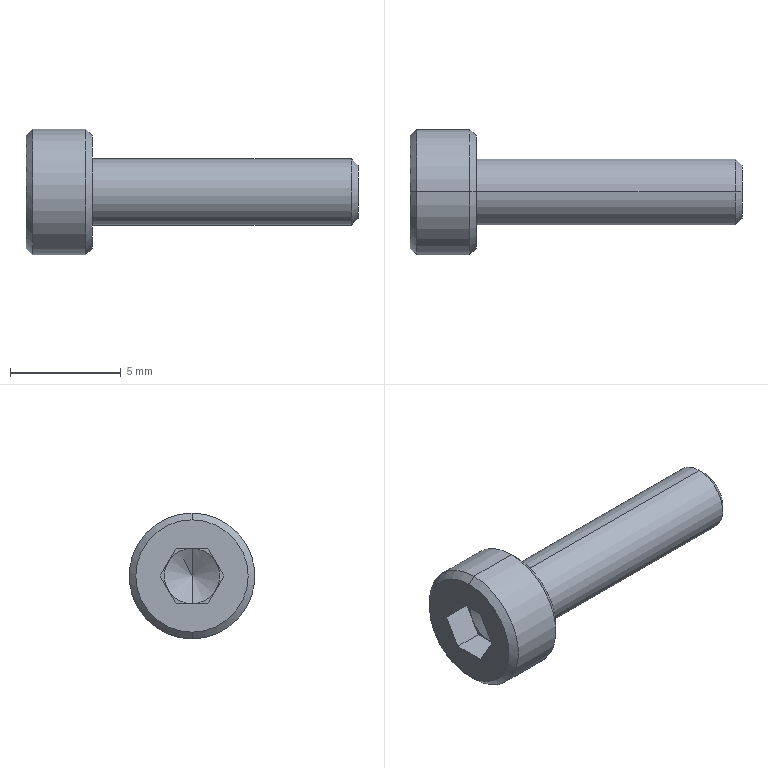Part | STEP file | Hex socket screw Dongming full thread M3-12 A2-70-1 | 1 solid | 27 faces | box 15 x 5.68 x 5.68 mm | volume 150.677 mm3 | plane 15 | cone 8 | cylinder 4 | commonest cylinder face diameters 3 x2 5.68 x2
STEP:
#1=CARTESIAN_POINT('',(15.,0.,-1.2));
#2=VERTEX_POINT('',#1);
#3=CARTESIAN_POINT('',(15.,0.,1.2));
#4=VERTEX_POINT('',#3);
#5=CARTESIAN_POINT('',(15.,0.,0.));
#6=DIRECTION('',(1.,0.,0.));
#7=DIRECTION('',(0.,0.,-1.));
#8=AXIS2_PLACEMENT_3D('',#5,#6,#7);
#9=CIRCLE('',#8,1.2);
#10=EDGE_CURVE('',#2,#4,#9,.T.);
#11=ORIENTED_EDGE('',*,*,#10,.F.);
#12=CARTESIAN_POINT('',(14.7,0.,-1.5));
#13=VERTEX_POINT('',#12);
#14=CARTESIAN_POINT('',(15.,0.,-1.2));
#15=DIRECTION('',(-0.7071,0.,-0.7071));
#16=VECTOR('',#15,1000.);
#17=LINE('',#14,#16);
#18=EDGE_CURVE('',#2,#13,#17,.T.);
#19=ORIENTED_EDGE('',*,*,#18,.T.);
#20=CARTESIAN_POINT('',(14.7,0.,1.5));
#21=VERTEX_POINT('',#20);
#22=CARTESIAN_POINT('',(14.7,0.,0.));
#23=DIRECTION('',(-1.,0.,0.));
#24=DIRECTION('',(0.,0.,-1.));
#25=AXIS2_PLACEMENT_3D('',#22,#23,#24);
#26=CIRCLE('',#25,1.5);
#27=EDGE_CURVE('',#21,#13,#26,.T.);
#28=ORIENTED_EDGE('',*,*,#27,.F.);
#29=CARTESIAN_POINT('',(15.,0.,1.2));
#30=DIRECTION('',(-0.7071,0.,0.7071));
#31=VECTOR('',#30,1000.);
#32=LINE('',#29,#31);
#33=EDGE_CURVE('',#4,#21,#32,.T.);
#34=ORIENTED_EDGE('',*,*,#33,.F.);
#35=EDGE_LOOP('',(#11,#19,#28,#34));
#36=FACE_OUTER_BOUND('',#35,.T.);
#37=CARTESIAN_POINT('',(15.,0.,0.));
#38=DIRECTION('',(-1.,0.,0.));
#39=DIRECTION('',(0.,0.,1.));
#40=AXIS2_PLACEMENT_3D('',#37,#38,#39);
#41=CONICAL_SURFACE('',#40,1.2,0.7854);
#42=ADVANCED_FACE('',(#36),#41,.T.);
#43=CARTESIAN_POINT('',(3.,0.,-2.54));
#44=VERTEX_POINT('',#43);
#45=CARTESIAN_POINT('',(3.,0.,2.54));
#46=VERTEX_POINT('',#45);
#47=CARTESIAN_POINT('',(3.,0.,0.));
#48=DIRECTION('',(1.,0.,0.));
#49=DIRECTION('',(0.,0.,-1.));
#50=AXIS2_PLACEMENT_3D('',#47,#48,#49);
#51=CIRCLE('',#50,2.54);
#52=EDGE_CURVE('',#44,#46,#51,.T.);
#53=ORIENTED_EDGE('',*,*,#52,.F.);
#54=CARTESIAN_POINT('',(2.7,0.,-2.84));
#55=VERTEX_POINT('',#54);
#56=CARTESIAN_POINT('',(3.,0.,-2.54));
#57=DIRECTION('',(-0.7071,0.,-0.7071));
#58=VECTOR('',#57,1000.);
#59=LINE('',#56,#58);
#60=EDGE_CURVE('',#44,#55,#59,.T.);
#61=ORIENTED_EDGE('',*,*,#60,.T.);
#62=CARTESIAN_POINT('',(2.7,0.,2.84));
#63=VERTEX_POINT('',#62);
#64=CARTESIAN_POINT('',(2.7,0.,0.));
#65=DIRECTION('',(-1.,0.,0.));
#66=DIRECTION('',(0.,0.,-1.));
#67=AXIS2_PLACEMENT_3D('',#64,#65,#66);
#68=CIRCLE('',#67,2.84);
#69=EDGE_CURVE('',#63,#55,#68,.T.);
#70=ORIENTED_EDGE('',*,*,#69,.F.);
#71=CARTESIAN_POINT('',(3.,0.,2.54));
#72=DIRECTION('',(-0.7071,0.,0.7071));
#73=VECTOR('',#72,1000.);
#74=LINE('',#71,#73);
#75=EDGE_CURVE('',#46,#63,#74,.T.);
#76=ORIENTED_EDGE('',*,*,#75,.F.);
#77=EDGE_LOOP('',(#53,#61,#70,#76));
#78=FACE_OUTER_BOUND('',#77,.T.);
#79=CARTESIAN_POINT('',(3.,0.,0.));
#80=DIRECTION('',(-1.,0.,0.));
#81=DIRECTION('',(0.,0.,1.));
#82=AXIS2_PLACEMENT_3D('',#79,#80,#81);
#83=CONICAL_SURFACE('',#82,2.54,0.7854);
#84=ADVANCED_FACE('',(#78),#83,.T.);
#85=CARTESIAN_POINT('',(0.,0.,2.54));
#86=VERTEX_POINT('',#85);
#87=CARTESIAN_POINT('',(0.,0.,-2.54));
#88=VERTEX_POINT('',#87);
#89=CARTESIAN_POINT('',(0.,0.,0.));
#90=DIRECTION('',(-1.,0.,0.));
#91=DIRECTION('',(0.,0.,-1.));
#92=AXIS2_PLACEMENT_3D('',#89,#90,#91);
#93=CIRCLE('',#92,2.54);
#94=EDGE_CURVE('',#86,#88,#93,.T.);
#95=ORIENTED_EDGE('',*,*,#94,.F.);
#96=CARTESIAN_POINT('',(0.3,0.,2.84));
#97=VERTEX_POINT('',#96);
#98=CARTESIAN_POINT('',(0.3,0.,2.84));
#99=DIRECTION('',(0.7071,0.,0.7071));
#100=VECTOR('',#99,1000.);
#101=LINE('',#98,#100);
#102=EDGE_CURVE('',#86,#97,#101,.T.);
#103=ORIENTED_EDGE('',*,*,#102,.T.);
#104=CARTESIAN_POINT('',(0.3,0.,-2.84));
#105=VERTEX_POINT('',#104);
#106=CARTESIAN_POINT('',(0.3,0.,0.));
#107=DIRECTION('',(1.,0.,0.));
#108=DIRECTION('',(0.,0.,-1.));
#109=AXIS2_PLACEMENT_3D('',#106,#107,#108);
#110=CIRCLE('',#109,2.84);
#111=EDGE_CURVE('',#105,#97,#110,.T.);
#112=ORIENTED_EDGE('',*,*,#111,.F.);
#113=CARTESIAN_POINT('',(0.3,0.,-2.84));
#114=DIRECTION('',(0.7071,0.,-0.7071));
#115=VECTOR('',#114,1000.);
#116=LINE('',#113,#115);
#117=EDGE_CURVE('',#88,#105,#116,.T.);
#118=ORIENTED_EDGE('',*,*,#117,.F.);
#119=EDGE_LOOP('',(#95,#103,#112,#118));
#120=FACE_OUTER_BOUND('',#119,.T.);
#121=CARTESIAN_POINT('',(0.3,0.,0.));
#122=DIRECTION('',(1.,0.,0.));
#123=DIRECTION('',(0.,0.,-1.));
#124=AXIS2_PLACEMENT_3D('',#121,#122,#123);
#125=CONICAL_SURFACE('',#124,2.84,0.7854);
#126=ADVANCED_FACE('',(#120),#125,.T.);
#127=CARTESIAN_POINT('',(2.022,0.,0.));
#128=VERTEX_POINT('',#127);
#129=CARTESIAN_POINT('',(1.3,0.,1.25));
#130=VERTEX_POINT('',#129);
#131=CARTESIAN_POINT('',(2.022,0.,0.));
#132=DIRECTION('',(-0.5,0.,0.866));
#133=VECTOR('',#132,1000.);
#134=LINE('',#131,#133);
#135=EDGE_CURVE('',#128,#130,#134,.T.);
#136=ORIENTED_EDGE('',*,*,#135,.F.);
#137=CARTESIAN_POINT('',(1.3,0.,-1.25));
#138=VERTEX_POINT('',#137);
#139=CARTESIAN_POINT('',(2.022,0.,0.));
#140=DIRECTION('',(-0.5,0.,-0.866));
#141=VECTOR('',#140,1000.);
#142=LINE('',#139,#141);
#143=EDGE_CURVE('',#128,#138,#142,.T.);
#144=ORIENTED_EDGE('',*,*,#143,.T.);
#145=CARTESIAN_POINT('',(1.3,-1.083,-0.625));
#146=VERTEX_POINT('',#145);
#147=CARTESIAN_POINT('',(1.3,0.,0.));
#148=DIRECTION('',(-1.,0.,0.));
#149=DIRECTION('',(0.,0.,1.));
#150=AXIS2_PLACEMENT_3D('',#147,#148,#149);
#151=CIRCLE('',#150,1.25);
#152=EDGE_CURVE('',#138,#146,#151,.T.);
#153=ORIENTED_EDGE('',*,*,#152,.T.);
#154=CARTESIAN_POINT('',(1.3,-1.083,0.625));
#155=VERTEX_POINT('',#154);
#156=CARTESIAN_POINT('',(1.3,0.,0.));
#157=DIRECTION('',(-1.,0.,0.));
#158=DIRECTION('',(0.,0.,1.));
#159=AXIS2_PLACEMENT_3D('',#156,#157,#158);
#160=CIRCLE('',#159,1.25);
#161=EDGE_CURVE('',#146,#155,#160,.T.);
#162=ORIENTED_EDGE('',*,*,#161,.T.);
#163=CARTESIAN_POINT('',(1.3,0.,0.));
#164=DIRECTION('',(-1.,0.,0.));
#165=DIRECTION('',(0.,0.,1.));
#166=AXIS2_PLACEMENT_3D('',#163,#164,#165);
#167=CIRCLE('',#166,1.25);
#168=EDGE_CURVE('',#155,#130,#167,.T.);
#169=ORIENTED_EDGE('',*,*,#168,.T.);
#170=EDGE_LOOP('',(#136,#144,#153,#162,#169));
#171=FACE_OUTER_BOUND('',#170,.T.);
#172=CARTESIAN_POINT('',(-997.978,0.,0.));
#173=DIRECTION('',(-1.,0.,0.));
#174=DIRECTION('',(0.,0.,1.));
#175=AXIS2_PLACEMENT_3D('',#172,#173,#174);
#176=CONICAL_SURFACE('',#175,1732.051,1.047);
#177=ADVANCED_FACE('',(#171),#176,.F.);
#178=ORIENTED_EDGE('',*,*,#27,.T.);
#179=CARTESIAN_POINT('',(3.,0.,-1.5));
#180=VERTEX_POINT('',#179);
#181=CARTESIAN_POINT('',(15.,0.,-1.5));
#182=DIRECTION('',(-1.,0.,0.));
#183=VECTOR('',#182,1000.);
#184=LINE('',#181,#183);
#185=EDGE_CURVE('',#13,#180,#184,.T.);
#186=ORIENTED_EDGE('',*,*,#185,.T.);
#187=CARTESIAN_POINT('',(3.,0.,1.5));
#188=VERTEX_POINT('',#187);
#189=CARTESIAN_POINT('',(3.,0.,0.));
#190=DIRECTION('',(1.,0.,0.));
#191=DIRECTION('',(0.,0.,-1.));
#192=AXIS2_PLACEMENT_3D('',#189,#190,#191);
#193=CIRCLE('',#192,1.5);
#194=EDGE_CURVE('',#180,#188,#193,.T.);
#195=ORIENTED_EDGE('',*,*,#194,.T.);
#196=CARTESIAN_POINT('',(15.,0.,1.5));
#197=DIRECTION('',(-1.,0.,0.));
#198=VECTOR('',#197,1000.);
#199=LINE('',#196,#198);
#200=EDGE_CURVE('',#21,#188,#199,.T.);
#201=ORIENTED_EDGE('',*,*,#200,.F.);
#202=EDGE_LOOP('',(#178,#186,#195,#201));
#203=FACE_OUTER_BOUND('',#202,.T.);
#204=CARTESIAN_POINT('',(15.,0.,0.));
#205=DIRECTION('',(-1.,0.,0.));
#206=DIRECTION('',(0.,0.,1.));
#207=AXIS2_PLACEMENT_3D('',#204,#205,#206);
#208=CYLINDRICAL_SURFACE('',#207,1.5);
#209=ADVANCED_FACE('',(#203),#208,.T.);
#210=ORIENTED_EDGE('',*,*,#69,.T.);
#211=CARTESIAN_POINT('',(3.,0.,-2.84));
#212=DIRECTION('',(-1.,0.,0.));
#213=VECTOR('',#212,1000.);
#214=LINE('',#211,#213);
#215=EDGE_CURVE('',#55,#105,#214,.T.);
#216=ORIENTED_EDGE('',*,*,#215,.T.);
#217=ORIENTED_EDGE('',*,*,#111,.T.);
#218=CARTESIAN_POINT('',(3.,0.,2.84));
#219=DIRECTION('',(-1.,0.,0.));
#220=VECTOR('',#219,1000.);
#221=LINE('',#218,#220);
#222=EDGE_CURVE('',#63,#97,#221,.T.);
#223=ORIENTED_EDGE('',*,*,#222,.F.);
#224=EDGE_LOOP('',(#210,#216,#217,#223));
#225=FACE_OUTER_BOUND('',#224,.T.);
#226=CARTESIAN_POINT('',(3.,0.,0.));
#227=DIRECTION('',(-1.,0.,0.));
#228=DIRECTION('',(0.,0.,1.));
#229=AXIS2_PLACEMENT_3D('',#226,#227,#228);
#230=CYLINDRICAL_SURFACE('',#229,2.84);
#231=ADVANCED_FACE('',(#225),#230,.T.);
#232=CARTESIAN_POINT('',(1.3,1.083,0.625));
#233=VERTEX_POINT('',#232);
#234=CARTESIAN_POINT('',(1.3,0.,0.));
#235=DIRECTION('',(-1.,0.,0.));
#236=DIRECTION('',(0.,0.,1.));
#237=AXIS2_PLACEMENT_3D('',#234,#235,#236);
#238=CIRCLE('',#237,1.25);
#239=EDGE_CURVE('',#130,#233,#238,.T.);
#240=ORIENTED_EDGE('',*,*,#239,.F.);
#241=CARTESIAN_POINT('',(1.3,0.7217,1.25));
#242=VERTEX_POINT('',#241);
#243=CARTESIAN_POINT('',(1.3,-0.7217,1.25));
#244=DIRECTION('',(0.,1.,0.));
#245=VECTOR('',#244,1000.);
#246=LINE('',#243,#245);
#247=EDGE_CURVE('',#130,#242,#246,.T.);
#248=ORIENTED_EDGE('',*,*,#247,.T.);
#249=CARTESIAN_POINT('',(1.3,0.7217,1.25));
#250=DIRECTION('',(0.,0.5,-0.866));
#251=VECTOR('',#250,1000.);
#252=LINE('',#249,#251);
#253=EDGE_CURVE('',#242,#233,#252,.T.);
#254=ORIENTED_EDGE('',*,*,#253,.T.);
#255=EDGE_LOOP('',(#240,#248,#254));
#256=FACE_OUTER_BOUND('',#255,.T.);
#257=CARTESIAN_POINT('',(1.3,0.,0.));
#258=DIRECTION('',(-1.,0.,0.));
#259=DIRECTION('',(0.,0.,1.));
#260=AXIS2_PLACEMENT_3D('',#257,#258,#259);
#261=PLANE('',#260);
#262=ADVANCED_FACE('',(#256),#261,.T.);
#263=CARTESIAN_POINT('',(1.3,1.083,-0.625));
#264=VERTEX_POINT('',#263);
#265=CARTESIAN_POINT('',(1.3,0.,0.));
#266=DIRECTION('',(-1.,0.,0.));
#267=DIRECTION('',(0.,0.,1.));
#268=AXIS2_PLACEMENT_3D('',#265,#266,#267);
#269=CIRCLE('',#268,1.25);
#270=EDGE_CURVE('',#233,#264,#269,.T.);
#271=ORIENTED_EDGE('',*,*,#270,.F.);
#272=CARTESIAN_POINT('',(1.3,1.443,0.));
#273=VERTEX_POINT('',#272);
#274=CARTESIAN_POINT('',(1.3,0.7217,1.25));
#275=DIRECTION('',(0.,0.5,-0.866));
#276=VECTOR('',#275,1000.);
#277=LINE('',#274,#276);
#278=EDGE_CURVE('',#233,#273,#277,.T.);
#279=ORIENTED_EDGE('',*,*,#278,.T.);
#280=CARTESIAN_POINT('',(1.3,1.443,0.));
#281=DIRECTION('',(0.,-0.5,-0.866));
#282=VECTOR('',#281,1000.);
#283=LINE('',#280,#282);
#284=EDGE_CURVE('',#273,#264,#283,.T.);
#285=ORIENTED_EDGE('',*,*,#284,.T.);
#286=EDGE_LOOP('',(#271,#279,#285));
#287=FACE_OUTER_BOUND('',#286,.T.);
#288=CARTESIAN_POINT('',(1.3,0.,0.));
#289=DIRECTION('',(-1.,0.,0.));
#290=DIRECTION('',(0.,0.,1.));
#291=AXIS2_PLACEMENT_3D('',#288,#289,#290);
#292=PLANE('',#291);
#293=ADVANCED_FACE('',(#287),#292,.T.);
#294=CARTESIAN_POINT('',(1.3,0.,0.));
#295=DIRECTION('',(-1.,0.,0.));
#296=DIRECTION('',(0.,0.,1.));
#297=AXIS2_PLACEMENT_3D('',#294,#295,#296);
#298=CIRCLE('',#297,1.25);
#299=EDGE_CURVE('',#264,#138,#298,.T.);
#300=ORIENTED_EDGE('',*,*,#299,.F.);
#301=CARTESIAN_POINT('',(1.3,0.7217,-1.25));
#302=VERTEX_POINT('',#301);
#303=CARTESIAN_POINT('',(1.3,1.443,0.));
#304=DIRECTION('',(0.,-0.5,-0.866));
#305=VECTOR('',#304,1000.);
#306=LINE('',#303,#305);
#307=EDGE_CURVE('',#264,#302,#306,.T.);
#308=ORIENTED_EDGE('',*,*,#307,.T.);
#309=CARTESIAN_POINT('',(1.3,0.7217,-1.25));
#310=DIRECTION('',(0.,-1.,0.));
#311=VECTOR('',#310,1000.);
#312=LINE('',#309,#311);
#313=EDGE_CURVE('',#302,#138,#312,.T.);
#314=ORIENTED_EDGE('',*,*,#313,.T.);
#315=EDGE_LOOP('',(#300,#308,#314));
#316=FACE_OUTER_BOUND('',#315,.T.);
#317=CARTESIAN_POINT('',(1.3,0.,0.));
#318=DIRECTION('',(-1.,0.,0.));
#319=DIRECTION('',(0.,0.,1.));
#320=AXIS2_PLACEMENT_3D('',#317,#318,#319);
#321=PLANE('',#320);
#322=ADVANCED_FACE('',(#316),#321,.T.);
#323=ORIENTED_EDGE('',*,*,#152,.F.);
#324=CARTESIAN_POINT('',(1.3,-0.7217,-1.25));
#325=VERTEX_POINT('',#324);
#326=CARTESIAN_POINT('',(1.3,0.7217,-1.25));
#327=DIRECTION('',(0.,-1.,0.));
#328=VECTOR('',#327,1000.);
#329=LINE('',#326,#328);
#330=EDGE_CURVE('',#138,#325,#329,.T.);
#331=ORIENTED_EDGE('',*,*,#330,.T.);
#332=CARTESIAN_POINT('',(1.3,-0.7217,-1.25));
#333=DIRECTION('',(0.,-0.5,0.866));
#334=VECTOR('',#333,1000.);
#335=LINE('',#332,#334);
#336=EDGE_CURVE('',#325,#146,#335,.T.);
#337=ORIENTED_EDGE('',*,*,#336,.T.);
#338=EDGE_LOOP('',(#323,#331,#337));
#339=FACE_OUTER_BOUND('',#338,.T.);
#340=CARTESIAN_POINT('',(1.3,0.,0.));
#341=DIRECTION('',(-1.,0.,0.));
#342=DIRECTION('',(0.,0.,1.));
#343=AXIS2_PLACEMENT_3D('',#340,#341,#342);
#344=PLANE('',#343);
#345=ADVANCED_FACE('',(#339),#344,.T.);
#346=ORIENTED_EDGE('',*,*,#161,.F.);
#347=CARTESIAN_POINT('',(1.3,-1.443,0.));
#348=VERTEX_POINT('',#347);
#349=CARTESIAN_POINT('',(1.3,-0.7217,-1.25));
#350=DIRECTION('',(0.,-0.5,0.866));
#351=VECTOR('',#350,1000.);
#352=LINE('',#349,#351);
#353=EDGE_CURVE('',#146,#348,#352,.T.);
#354=ORIENTED_EDGE('',*,*,#353,.T.);
#355=CARTESIAN_POINT('',(1.3,-1.443,0.));
#356=DIRECTION('',(0.,0.5,0.866));
#357=VECTOR('',#356,1000.);
#358=LINE('',#355,#357);
#359=EDGE_CURVE('',#348,#155,#358,.T.);
#360=ORIENTED_EDGE('',*,*,#359,.T.);
#361=EDGE_LOOP('',(#346,#354,#360));
#362=FACE_OUTER_BOUND('',#361,.T.);
#363=CARTESIAN_POINT('',(1.3,0.,0.));
#364=DIRECTION('',(-1.,0.,0.));
#365=DIRECTION('',(0.,0.,1.));
#366=AXIS2_PLACEMENT_3D('',#363,#364,#365);
#367=PLANE('',#366);
#368=ADVANCED_FACE('',(#362),#367,.T.);
#369=ORIENTED_EDGE('',*,*,#215,.F.);
#370=CARTESIAN_POINT('',(2.7,0.,0.));
#371=DIRECTION('',(-1.,0.,0.));
#372=DIRECTION('',(0.,0.,-1.));
#373=AXIS2_PLACEMENT_3D('',#370,#371,#372);
#374=CIRCLE('',#373,2.84);
#375=EDGE_CURVE('',#55,#63,#374,.T.);
#376=ORIENTED_EDGE('',*,*,#375,.T.);
#377=ORIENTED_EDGE('',*,*,#222,.T.);
#378=CARTESIAN_POINT('',(0.3,0.,0.));
#379=DIRECTION('',(1.,0.,0.));
#380=DIRECTION('',(0.,0.,-1.));
#381=AXIS2_PLACEMENT_3D('',#378,#379,#380);
#382=CIRCLE('',#381,2.84);
#383=EDGE_CURVE('',#97,#105,#382,.T.);
#384=ORIENTED_EDGE('',*,*,#383,.T.);
#385=EDGE_LOOP('',(#369,#376,#377,#384));
#386=FACE_OUTER_BOUND('',#385,.T.);
#387=CARTESIAN_POINT('',(3.,0.,0.));
#388=DIRECTION('',(-1.,0.,0.));
#389=DIRECTION('',(0.,0.,1.));
#390=AXIS2_PLACEMENT_3D('',#387,#388,#389);
#391=CYLINDRICAL_SURFACE('',#390,2.84);
#392=ADVANCED_FACE('',(#386),#391,.T.);
#393=CARTESIAN_POINT('',(3.,0.,0.));
#394=DIRECTION('',(1.,0.,0.));
#395=DIRECTION('',(0.,0.,-1.));
#396=AXIS2_PLACEMENT_3D('',#393,#394,#395);
#397=CIRCLE('',#396,2.54);
#398=EDGE_CURVE('',#46,#44,#397,.T.);
#399=ORIENTED_EDGE('',*,*,#398,.T.);
#400=ORIENTED_EDGE('',*,*,#52,.T.);
#401=EDGE_LOOP('',(#399,#400));
#402=FACE_OUTER_BOUND('',#401,.T.);
#403=CARTESIAN_POINT('',(3.,0.,0.));
#404=DIRECTION('',(1.,0.,0.));
#405=DIRECTION('',(0.,0.,-1.));
#406=AXIS2_PLACEMENT_3D('',#403,#404,#405);
#407=CIRCLE('',#406,1.5);
#408=EDGE_CURVE('',#188,#180,#407,.T.);
#409=ORIENTED_EDGE('',*,*,#408,.F.);
#410=ORIENTED_EDGE('',*,*,#194,.F.);
#411=EDGE_LOOP('',(#409,#410));
#412=FACE_BOUND('',#411,.T.);
#413=CARTESIAN_POINT('',(3.,0.,0.));
#414=DIRECTION('',(1.,0.,0.));
#415=DIRECTION('',(0.,0.,-1.));
#416=AXIS2_PLACEMENT_3D('',#413,#414,#415);
#417=PLANE('',#416);
#418=ADVANCED_FACE('',(#402,#412),#417,.T.);
#419=CARTESIAN_POINT('',(0.,0.,0.));
#420=DIRECTION('',(-1.,0.,0.));
#421=DIRECTION('',(0.,0.,-1.));
#422=AXIS2_PLACEMENT_3D('',#419,#420,#421);
#423=CIRCLE('',#422,2.54);
#424=EDGE_CURVE('',#88,#86,#423,.T.);
#425=ORIENTED_EDGE('',*,*,#424,.T.);
#426=ORIENTED_EDGE('',*,*,#94,.T.);
#427=EDGE_LOOP('',(#425,#426));
#428=FACE_OUTER_BOUND('',#427,.T.);
#429=CARTESIAN_POINT('',(0.,1.443,0.));
#430=VERTEX_POINT('',#429);
#431=CARTESIAN_POINT('',(0.,0.7217,-1.25));
#432=VERTEX_POINT('',#431);
#433=CARTESIAN_POINT('',(0.,1.443,0.));
#434=DIRECTION('',(0.,-0.5,-0.866));
#435=VECTOR('',#434,1000.);
#436=LINE('',#433,#435);
#437=EDGE_CURVE('',#430,#432,#436,.T.);
#438=ORIENTED_EDGE('',*,*,#437,.F.);
#439=CARTESIAN_POINT('',(0.,0.7217,1.25));
#440=VERTEX_POINT('',#439);
#441=CARTESIAN_POINT('',(0.,0.7217,1.25));
#442=DIRECTION('',(0.,0.5,-0.866));
#443=VECTOR('',#442,1000.);
#444=LINE('',#441,#443);
#445=EDGE_CURVE('',#440,#430,#444,.T.);
#446=ORIENTED_EDGE('',*,*,#445,.F.);
#447=CARTESIAN_POINT('',(0.,-0.7217,1.25));
#448=VERTEX_POINT('',#447);
#449=CARTESIAN_POINT('',(0.,-0.7217,1.25));
#450=DIRECTION('',(0.,1.,0.));
#451=VECTOR('',#450,1000.);
#452=LINE('',#449,#451);
#453=EDGE_CURVE('',#448,#440,#452,.T.);
#454=ORIENTED_EDGE('',*,*,#453,.F.);
#455=CARTESIAN_POINT('',(0.,-1.443,0.));
#456=VERTEX_POINT('',#455);
#457=CARTESIAN_POINT('',(0.,-1.443,0.));
#458=DIRECTION('',(0.,0.5,0.866));
#459=VECTOR('',#458,1000.);
#460=LINE('',#457,#459);
#461=EDGE_CURVE('',#456,#448,#460,.T.);
#462=ORIENTED_EDGE('',*,*,#461,.F.);
#463=CARTESIAN_POINT('',(0.,-0.7217,-1.25));
#464=VERTEX_POINT('',#463);
#465=CARTESIAN_POINT('',(0.,-0.7217,-1.25));
#466=DIRECTION('',(0.,-0.5,0.866));
#467=VECTOR('',#466,1000.);
#468=LINE('',#465,#467);
#469=EDGE_CURVE('',#464,#456,#468,.T.);
#470=ORIENTED_EDGE('',*,*,#469,.F.);
#471=CARTESIAN_POINT('',(0.,0.7217,-1.25));
#472=DIRECTION('',(0.,-1.,0.));
#473=VECTOR('',#472,1000.);
#474=LINE('',#471,#473);
#475=EDGE_CURVE('',#432,#464,#474,.T.);
#476=ORIENTED_EDGE('',*,*,#475,.F.);
#477=EDGE_LOOP('',(#438,#446,#454,#462,#470,#476));
#478=FACE_BOUND('',#477,.T.);
#479=CARTESIAN_POINT('',(0.,0.,0.));
#480=DIRECTION('',(1.,0.,0.));
#481=DIRECTION('',(0.,0.,-1.));
#482=AXIS2_PLACEMENT_3D('',#479,#480,#481);
#483=PLANE('',#482);
#484=ADVANCED_FACE('',(#428,#478),#483,.F.);
#485=ORIENTED_EDGE('',*,*,#185,.F.);
#486=CARTESIAN_POINT('',(14.7,0.,0.));
#487=DIRECTION('',(-1.,0.,0.));
#488=DIRECTION('',(0.,0.,-1.));
#489=AXIS2_PLACEMENT_3D('',#486,#487,#488);
#490=CIRCLE('',#489,1.5);
#491=EDGE_CURVE('',#13,#21,#490,.T.);
#492=ORIENTED_EDGE('',*,*,#491,.T.);
#493=ORIENTED_EDGE('',*,*,#200,.T.);
#494=ORIENTED_EDGE('',*,*,#408,.T.);
#495=EDGE_LOOP('',(#485,#492,#493,#494));
#496=FACE_OUTER_BOUND('',#495,.T.);
#497=CARTESIAN_POINT('',(15.,0.,0.));
#498=DIRECTION('',(-1.,0.,0.));
#499=DIRECTION('',(0.,0.,1.));
#500=AXIS2_PLACEMENT_3D('',#497,#498,#499);
#501=CYLINDRICAL_SURFACE('',#500,1.5);
#502=ADVANCED_FACE('',(#496),#501,.T.);
#503=CARTESIAN_POINT('',(15.,0.,0.));
#504=DIRECTION('',(1.,0.,0.));
#505=DIRECTION('',(0.,0.,-1.));
#506=AXIS2_PLACEMENT_3D('',#503,#504,#505);
#507=CIRCLE('',#506,1.2);
#508=EDGE_CURVE('',#4,#2,#507,.T.);
#509=ORIENTED_EDGE('',*,*,#508,.T.);
#510=ORIENTED_EDGE('',*,*,#10,.T.);
#511=EDGE_LOOP('',(#509,#510));
#512=FACE_OUTER_BOUND('',#511,.T.);
#513=CARTESIAN_POINT('',(15.,0.,0.));
#514=DIRECTION('',(1.,0.,0.));
#515=DIRECTION('',(0.,0.,-1.));
#516=AXIS2_PLACEMENT_3D('',#513,#514,#515);
#517=PLANE('',#516);
#518=ADVANCED_FACE('',(#512),#517,.T.);
#519=ORIENTED_EDGE('',*,*,#445,.T.);
#520=CARTESIAN_POINT('',(1.3,1.443,0.));
#521=DIRECTION('',(-1.,0.,0.));
#522=VECTOR('',#521,1000.);
#523=LINE('',#520,#522);
#524=EDGE_CURVE('',#273,#430,#523,.T.);
#525=ORIENTED_EDGE('',*,*,#524,.F.);
#526=ORIENTED_EDGE('',*,*,#278,.F.);
#527=ORIENTED_EDGE('',*,*,#253,.F.);
#528=CARTESIAN_POINT('',(1.3,0.7217,1.25));
#529=DIRECTION('',(-1.,0.,0.));
#530=VECTOR('',#529,1000.);
#531=LINE('',#528,#530);
#532=EDGE_CURVE('',#242,#440,#531,.T.);
#533=ORIENTED_EDGE('',*,*,#532,.T.);
#534=EDGE_LOOP('',(#519,#525,#526,#527,#533));
#535=FACE_OUTER_BOUND('',#534,.T.);
#536=CARTESIAN_POINT('',(1.3,0.7217,1.25));
#537=DIRECTION('',(0.,0.866,0.5));
#538=DIRECTION('',(0.,-0.5,0.866));
#539=AXIS2_PLACEMENT_3D('',#536,#537,#538);
#540=PLANE('',#539);
#541=ADVANCED_FACE('',(#535),#540,.F.);
#542=ORIENTED_EDGE('',*,*,#453,.T.);
#543=ORIENTED_EDGE('',*,*,#532,.F.);
#544=ORIENTED_EDGE('',*,*,#247,.F.);
#545=CARTESIAN_POINT('',(1.3,-0.7217,1.25));
#546=VERTEX_POINT('',#545);
#547=CARTESIAN_POINT('',(1.3,-0.7217,1.25));
#548=DIRECTION('',(0.,1.,0.));
#549=VECTOR('',#548,1000.);
#550=LINE('',#547,#549);
#551=EDGE_CURVE('',#546,#130,#550,.T.);
#552=ORIENTED_EDGE('',*,*,#551,.F.);
#553=CARTESIAN_POINT('',(1.3,-0.7217,1.25));
#554=DIRECTION('',(-1.,0.,0.));
#555=VECTOR('',#554,1000.);
#556=LINE('',#553,#555);
#557=EDGE_CURVE('',#546,#448,#556,.T.);
#558=ORIENTED_EDGE('',*,*,#557,.T.);
#559=EDGE_LOOP('',(#542,#543,#544,#552,#558));
#560=FACE_OUTER_BOUND('',#559,.T.);
#561=CARTESIAN_POINT('',(1.3,-0.7217,1.25));
#562=DIRECTION('',(0.,0.,1.));
#563=DIRECTION('',(0.,-1.,0.));
#564=AXIS2_PLACEMENT_3D('',#561,#562,#563);
#565=PLANE('',#564);
#566=ADVANCED_FACE('',(#560),#565,.F.);
#567=ORIENTED_EDGE('',*,*,#461,.T.);
#568=ORIENTED_EDGE('',*,*,#557,.F.);
#569=CARTESIAN_POINT('',(1.3,-1.443,0.));
#570=DIRECTION('',(0.,0.5,0.866));
#571=VECTOR('',#570,1000.);
#572=LINE('',#569,#571);
#573=EDGE_CURVE('',#155,#546,#572,.T.);
#574=ORIENTED_EDGE('',*,*,#573,.F.);
#575=ORIENTED_EDGE('',*,*,#359,.F.);
#576=CARTESIAN_POINT('',(1.3,-1.443,0.));
#577=DIRECTION('',(-1.,0.,0.));
#578=VECTOR('',#577,1000.);
#579=LINE('',#576,#578);
#580=EDGE_CURVE('',#348,#456,#579,.T.);
#581=ORIENTED_EDGE('',*,*,#580,.T.);
#582=EDGE_LOOP('',(#567,#568,#574,#575,#581));
#583=FACE_OUTER_BOUND('',#582,.T.);
#584=CARTESIAN_POINT('',(1.3,-1.443,0.));
#585=DIRECTION('',(0.,-0.866,0.5));
#586=DIRECTION('',(0.,-0.5,-0.866));
#587=AXIS2_PLACEMENT_3D('',#584,#585,#586);
#588=PLANE('',#587);
#589=ADVANCED_FACE('',(#583),#588,.F.);
#590=ORIENTED_EDGE('',*,*,#469,.T.);
#591=ORIENTED_EDGE('',*,*,#580,.F.);
#592=ORIENTED_EDGE('',*,*,#353,.F.);
#593=ORIENTED_EDGE('',*,*,#336,.F.);
#594=CARTESIAN_POINT('',(1.3,-0.7217,-1.25));
#595=DIRECTION('',(-1.,0.,0.));
#596=VECTOR('',#595,1000.);
#597=LINE('',#594,#596);
#598=EDGE_CURVE('',#325,#464,#597,.T.);
#599=ORIENTED_EDGE('',*,*,#598,.T.);
#600=EDGE_LOOP('',(#590,#591,#592,#593,#599));
#601=FACE_OUTER_BOUND('',#600,.T.);
#602=CARTESIAN_POINT('',(1.3,-0.7217,-1.25));
#603=DIRECTION('',(0.,-0.866,-0.5));
#604=DIRECTION('',(0.,0.5,-0.866));
#605=AXIS2_PLACEMENT_3D('',#602,#603,#604);
#606=PLANE('',#605);
#607=ADVANCED_FACE('',(#601),#606,.F.);
#608=ORIENTED_EDGE('',*,*,#475,.T.);
#609=ORIENTED_EDGE('',*,*,#598,.F.);
#610=ORIENTED_EDGE('',*,*,#330,.F.);
#611=ORIENTED_EDGE('',*,*,#313,.F.);
#612=CARTESIAN_POINT('',(1.3,0.7217,-1.25));
#613=DIRECTION('',(-1.,0.,0.));
#614=VECTOR('',#613,1000.);
#615=LINE('',#612,#614);
#616=EDGE_CURVE('',#302,#432,#615,.T.);
#617=ORIENTED_EDGE('',*,*,#616,.T.);
#618=EDGE_LOOP('',(#608,#609,#610,#611,#617));
#619=FACE_OUTER_BOUND('',#618,.T.);
#620=CARTESIAN_POINT('',(1.3,0.7217,-1.25));
#621=DIRECTION('',(0.,0.,-1.));
#622=DIRECTION('',(-1.,0.,0.));
#623=AXIS2_PLACEMENT_3D('',#620,#621,#622);
#624=PLANE('',#623);
#625=ADVANCED_FACE('',(#619),#624,.F.);
#626=ORIENTED_EDGE('',*,*,#437,.T.);
#627=ORIENTED_EDGE('',*,*,#616,.F.);
#628=ORIENTED_EDGE('',*,*,#307,.F.);
#629=ORIENTED_EDGE('',*,*,#284,.F.);
#630=ORIENTED_EDGE('',*,*,#524,.T.);
#631=EDGE_LOOP('',(#626,#627,#628,#629,#630));
#632=FACE_OUTER_BOUND('',#631,.T.);
#633=CARTESIAN_POINT('',(1.3,1.443,0.));
#634=DIRECTION('',(0.,0.866,-0.5));
#635=DIRECTION('',(0.,0.5,0.866));
#636=AXIS2_PLACEMENT_3D('',#633,#634,#635);
#637=PLANE('',#636);
#638=ADVANCED_FACE('',(#632),#637,.F.);
#639=ORIENTED_EDGE('',*,*,#168,.F.);
#640=ORIENTED_EDGE('',*,*,#573,.T.);
#641=ORIENTED_EDGE('',*,*,#551,.T.);
#642=EDGE_LOOP('',(#639,#640,#641));
#643=FACE_OUTER_BOUND('',#642,.T.);
#644=CARTESIAN_POINT('',(1.3,0.,0.));
#645=DIRECTION('',(-1.,0.,0.));
#646=DIRECTION('',(0.,0.,1.));
#647=AXIS2_PLACEMENT_3D('',#644,#645,#646);
#648=PLANE('',#647);
#649=ADVANCED_FACE('',(#643),#648,.T.);
#650=ORIENTED_EDGE('',*,*,#143,.F.);
#651=ORIENTED_EDGE('',*,*,#135,.T.);
#652=ORIENTED_EDGE('',*,*,#239,.T.);
#653=ORIENTED_EDGE('',*,*,#270,.T.);
#654=ORIENTED_EDGE('',*,*,#299,.T.);
#655=EDGE_LOOP('',(#650,#651,#652,#653,#654));
#656=FACE_OUTER_BOUND('',#655,.T.);
#657=CARTESIAN_POINT('',(-997.978,0.,0.));
#658=DIRECTION('',(-1.,0.,0.));
#659=DIRECTION('',(0.,0.,1.));
#660=AXIS2_PLACEMENT_3D('',#657,#658,#659);
#661=CONICAL_SURFACE('',#660,1732.051,1.047);
#662=ADVANCED_FACE('',(#656),#661,.F.);
#663=ORIENTED_EDGE('',*,*,#102,.F.);
#664=ORIENTED_EDGE('',*,*,#424,.F.);
#665=ORIENTED_EDGE('',*,*,#117,.T.);
#666=ORIENTED_EDGE('',*,*,#383,.F.);
#667=EDGE_LOOP('',(#663,#664,#665,#666));
#668=FACE_OUTER_BOUND('',#667,.T.);
#669=CARTESIAN_POINT('',(0.3,0.,0.));
#670=DIRECTION('',(1.,0.,0.));
#671=DIRECTION('',(0.,0.,-1.));
#672=AXIS2_PLACEMENT_3D('',#669,#670,#671);
#673=CONICAL_SURFACE('',#672,2.84,0.7854);
#674=ADVANCED_FACE('',(#668),#673,.T.);
#675=ORIENTED_EDGE('',*,*,#60,.F.);
#676=ORIENTED_EDGE('',*,*,#398,.F.);
#677=ORIENTED_EDGE('',*,*,#75,.T.);
#678=ORIENTED_EDGE('',*,*,#375,.F.);
#679=EDGE_LOOP('',(#675,#676,#677,#678));
#680=FACE_OUTER_BOUND('',#679,.T.);
#681=CARTESIAN_POINT('',(3.,0.,0.));
#682=DIRECTION('',(-1.,0.,0.));
#683=DIRECTION('',(0.,0.,1.));
#684=AXIS2_PLACEMENT_3D('',#681,#682,#683);
#685=CONICAL_SURFACE('',#684,2.54,0.7854);
#686=ADVANCED_FACE('',(#680),#685,.T.);
#687=ORIENTED_EDGE('',*,*,#18,.F.);
#688=ORIENTED_EDGE('',*,*,#508,.F.);
#689=ORIENTED_EDGE('',*,*,#33,.T.);
#690=ORIENTED_EDGE('',*,*,#491,.F.);
#691=EDGE_LOOP('',(#687,#688,#689,#690));
#692=FACE_OUTER_BOUND('',#691,.T.);
#693=CARTESIAN_POINT('',(15.,0.,0.));
#694=DIRECTION('',(-1.,0.,0.));
#695=DIRECTION('',(0.,0.,1.));
#696=AXIS2_PLACEMENT_3D('',#693,#694,#695);
#697=CONICAL_SURFACE('',#696,1.2,0.7854);
#698=ADVANCED_FACE('',(#692),#697,.T.);
#699=CLOSED_SHELL('',(#42,#84,#126,#177,#209,#231,#262,#293,#322,#345,#368,#392,#418,#484,#502,#518,#541,#566,#589,#607,#625,#638,#649,#662,#674,#686,#698));
#700=MANIFOLD_SOLID_BREP('',#699);
#701=CARTESIAN_POINT('',(0.,0.,0.));
#702=DIRECTION('',(0.,0.,1.));
#703=DIRECTION('',(1.,0.,0.));
#704=AXIS2_PLACEMENT_3D('',#701,#702,#703);
#705=(LENGTH_UNIT()NAMED_UNIT(*)SI_UNIT(.MILLI.,.METRE.));
#706=UNCERTAINTY_MEASURE_WITH_UNIT(LENGTH_MEASURE(0.00001),#705,'','');
#707=(NAMED_UNIT(*)PLANE_ANGLE_UNIT()SI_UNIT($,.RADIAN.));
#708=(NAMED_UNIT(*)SI_UNIT($,.STERADIAN.)SOLID_ANGLE_UNIT());
#709=(GEOMETRIC_REPRESENTATION_CONTEXT(3)GLOBAL_UNCERTAINTY_ASSIGNED_CONTEXT((#706))GLOBAL_UNIT_ASSIGNED_CONTEXT((#705,#707,#708))REPRESENTATION_CONTEXT('',''));
#710=ADVANCED_BREP_SHAPE_REPRESENTATION('',(#700,#704),#709);